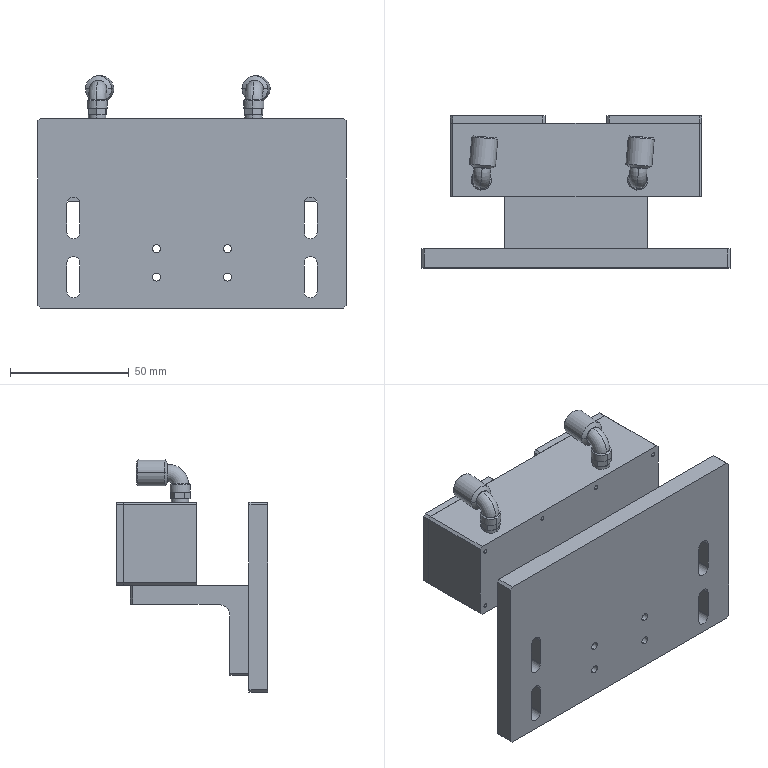Part | NX | features BREP 8 | 21 solids | 473 faces | box 130 x 64 x 97.9 mm | volume 230425 mm3 | cylinder 195 | plane 188 | cone 86 | torus 4 | commonest cylinder face diameters 3 x44 10 x27 5.5 x20 1.778 x16 3.1 x16 3.3 x16